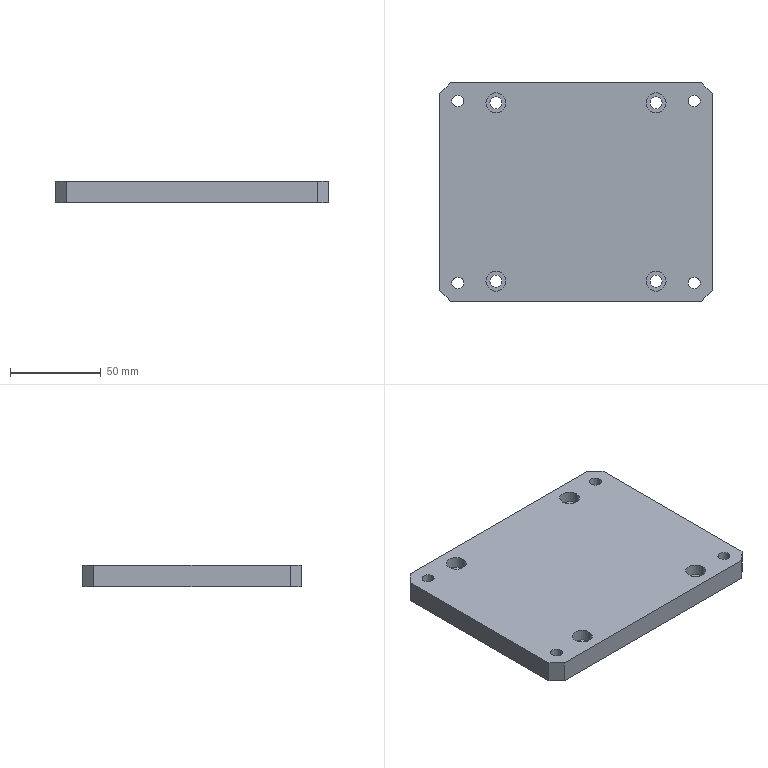Part | STEP file | 11-FG-E02311 | 1 solid | 62 faces | box 150 x 120 x 12 mm | volume 207598 mm3 | cylinder 40 | plane 22 | commonest cylinder face diameters 6.6 x16 11 x16 15 x8